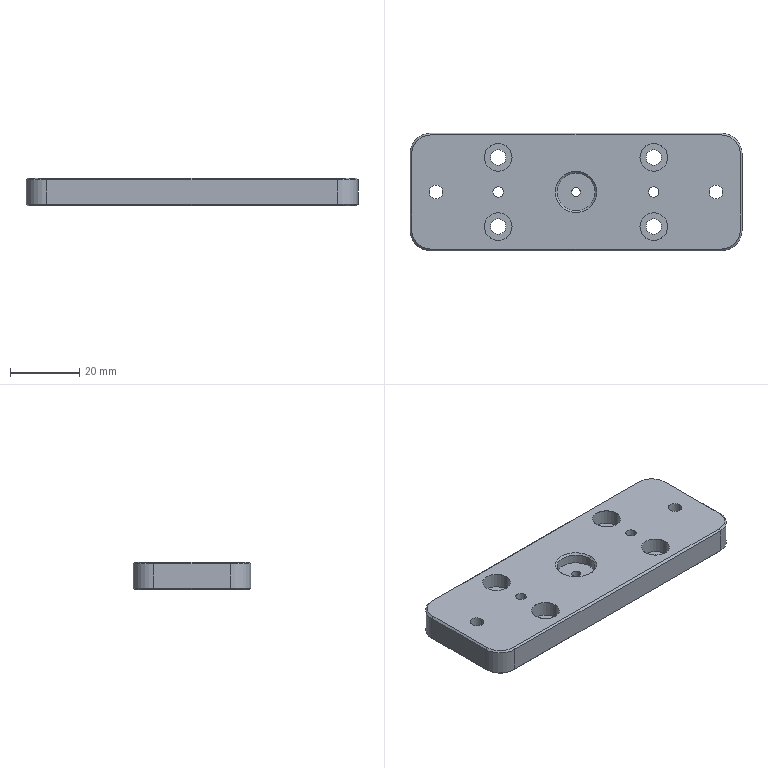Part | STEP file | QA-FB05 | 1 solid | 69 faces | box 96 x 34 x 8 mm | volume 24043 mm3 | cylinder 32 | plane 19 | cone 18 | commonest cylinder face diameters 4.5 x8 8 x8 3 x4 4 x4 12 x4 2.5 x2